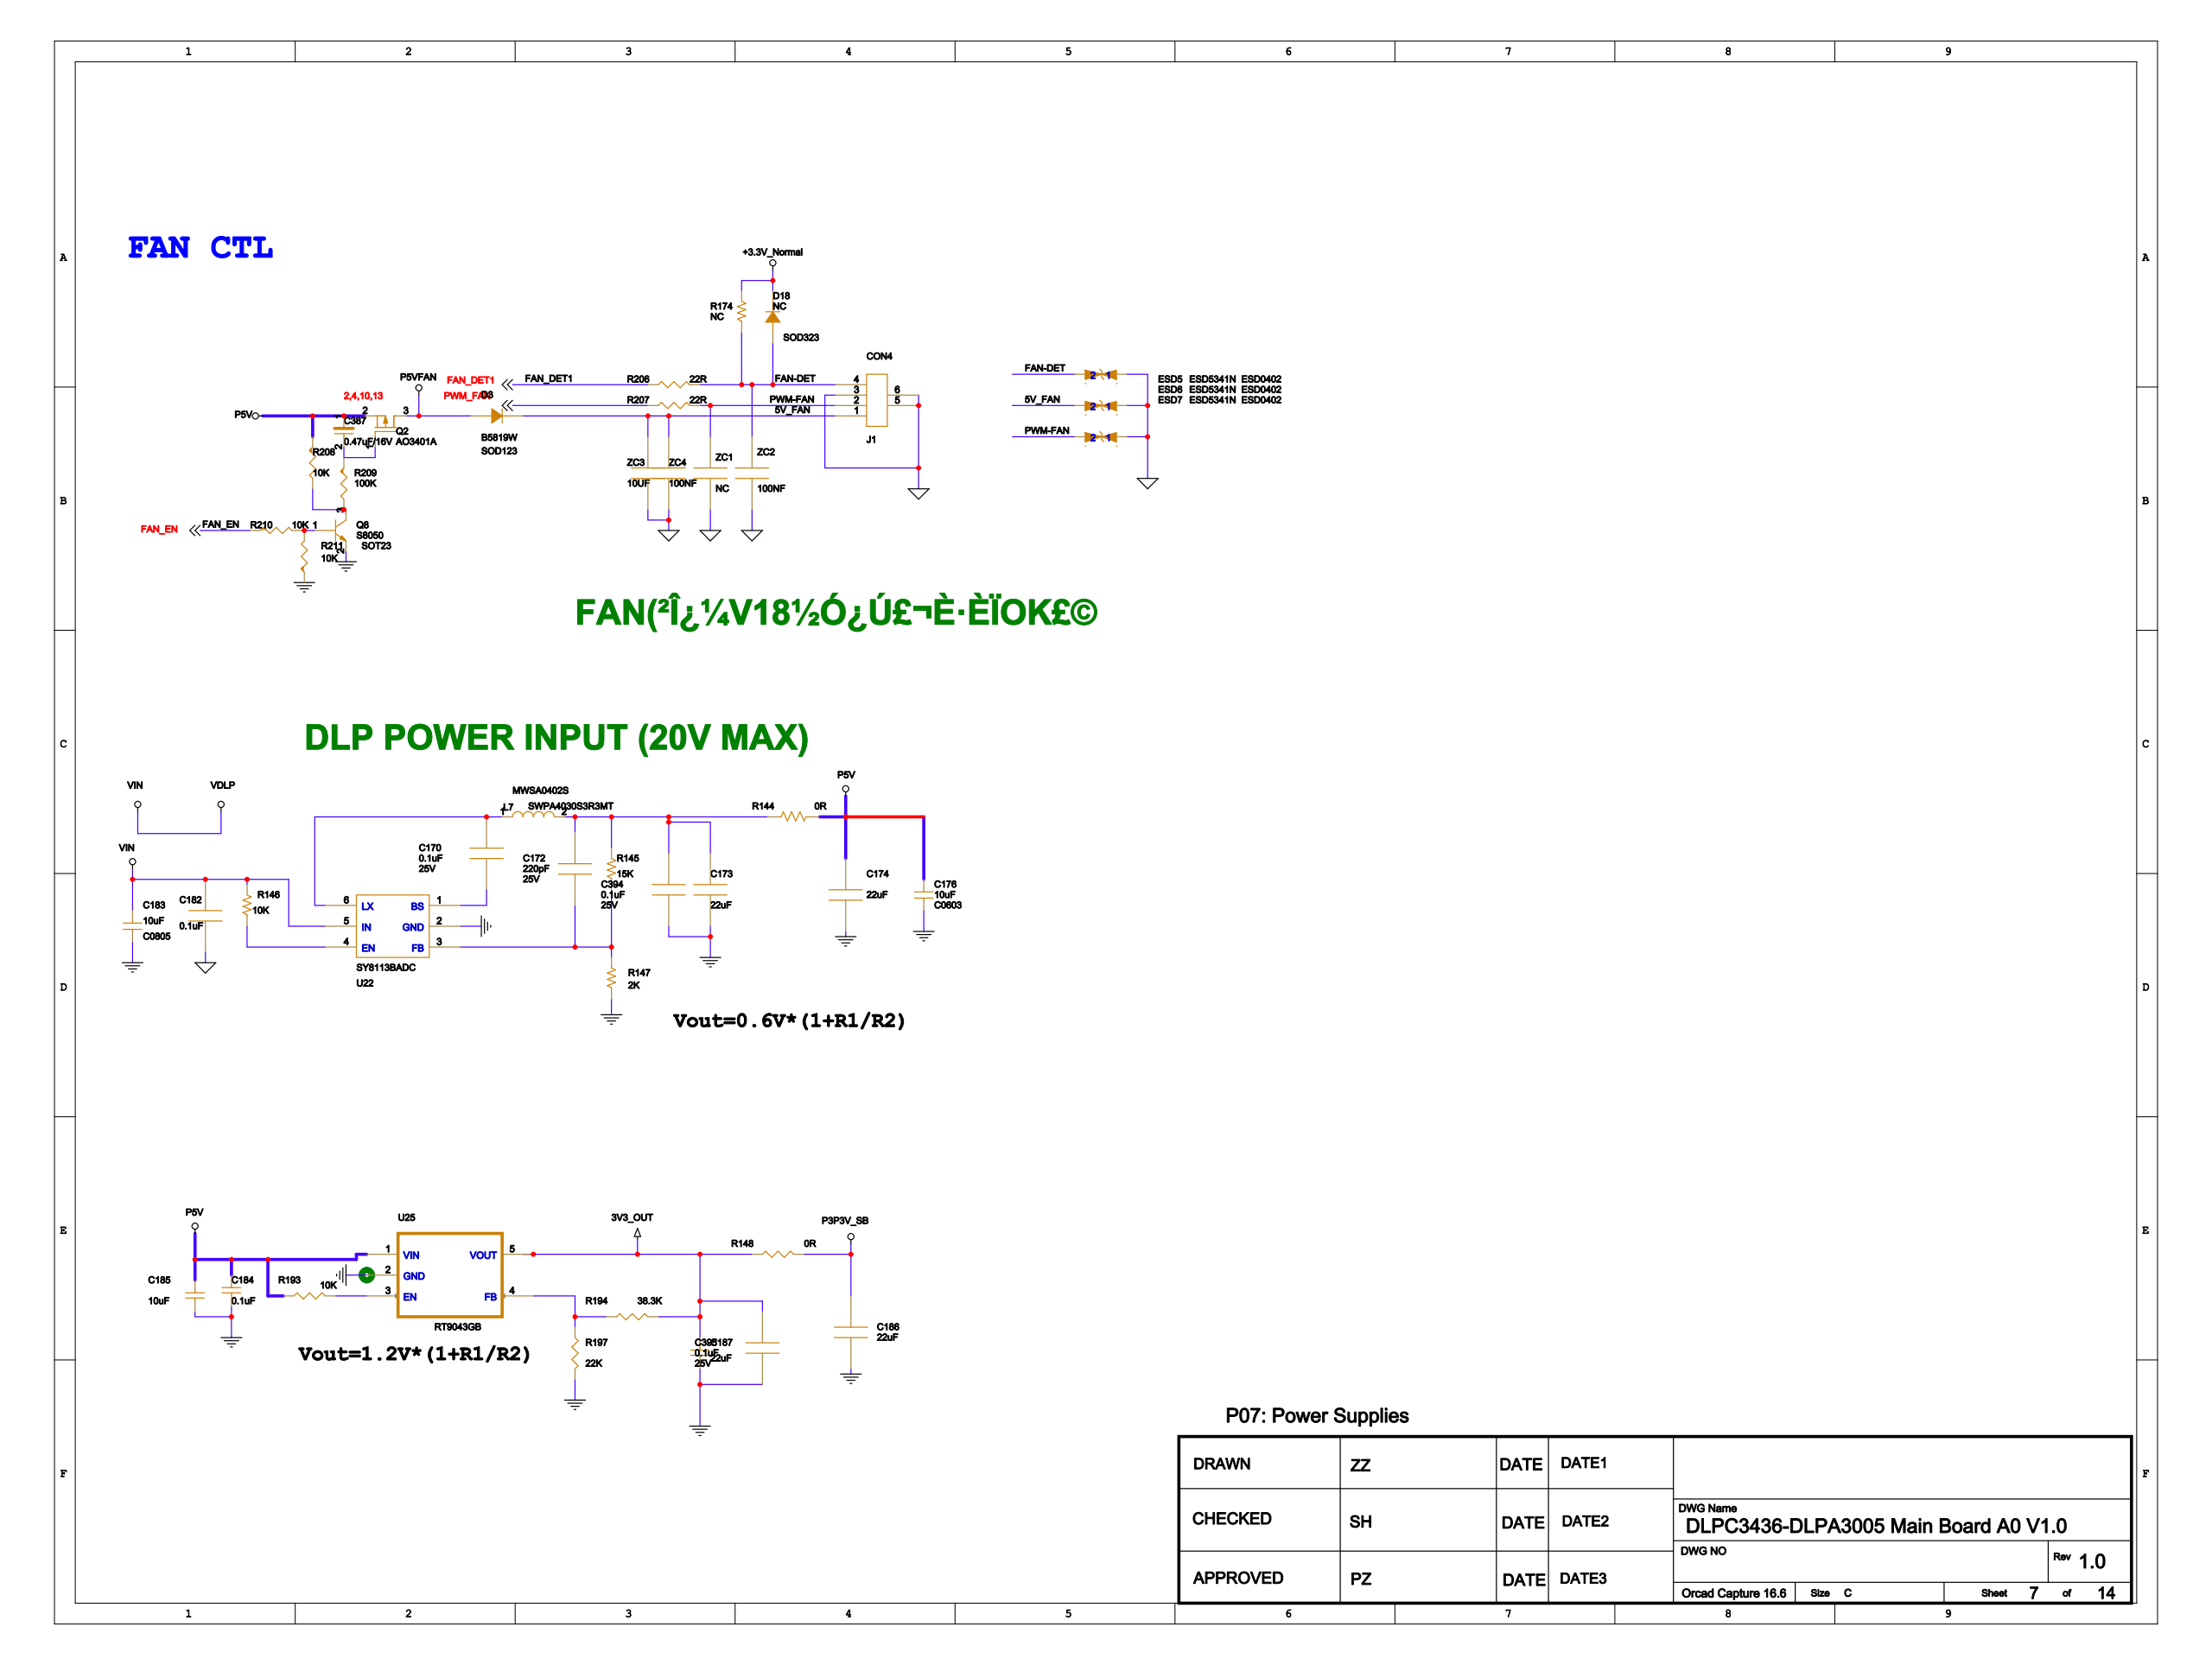Circuit board | Cadence Allegro | 1223 parts | 777 nets | one sheet of the schematic
Parts on this sheet (reference | value | footprint):
C170 | 0.1uF | C0402
C172 | 220pF | C0402
C173 | 22uF | C0603
C174 | 22uF | C0603
C176 | 10uF | C0603
C182 | 0.1uF | C0402
C183 | 10uF | C0805
C184 | 0.1uF | C0201
C185 | 10uF | C0603
C186 | 22uF | C0603
C187 | 22uF | C0603
C387 | 0.47uF/16V | C0402
C394 | 0.1uF | C0402
C395 | 0.1uF | C0402
D3 | B5819W | SOD123
D18 | NC | SOD323
ESD5 | ESD5341N | ESD0402
ESD6 | ESD5341N | ESD0402
ESD7 | ESD5341N | ESD0402
J1 | CON4 | CN1X4-1P25MM-WF
L7 | SWPA4030S3R3MT | MWSA0402S
Q2 | AO3401A | SOT23-100
Q8 | S8050 | SOT23
R144 | 0R | R0805
R145 | 15K | R0402
R146 | 10K | R0201
R147 | 2K | R0402
R148 | 0R | R0402
R174 | NC | R0402
R193 | 10K | R0201
R194 | 38.3K | R0402
R197 | 22K | R0402
R206 | 22R | R0402
R207 | 22R | R0402
R208 | 10K | R0402
R209 | 100K | R0402
R210 | 10K | R0402
R211 | 10K | R0402
U22 | SY8113BADC | SOT-23-6
U25 | RT9043GB | SOT25
ZC1 | NC | C0402
ZC2 | 100NF | C0402
ZC3 | 10uF | C0603
ZC4 | 100NF | C0402
Nets of these parts (net: part-pin ...):
GND: C173-2 C174-2 C176-1 C182-2 C183-1 C184-2 C185-2 C186-2 C187-2 C394-2 C395-2 ESD5-1 ESD6-1 ESD7-1 J1-3 J1-5 J1-6 Q8-2 R147-1 R197-2 R211-1 U22-2 U25-2 ZC1-1 ZC2-1 ZC3-1 ZC4-1
P3P3V_SB: C186-1 R148-2
VDLP: C182-1 C183-2 R146-2 U22-5
N23821148: C170-2 U22-1
N23821156: C170-1 L7-1 U22-6
N23821150: C172-1 C173-1 C394-1 L7-2 R144-1 R145-2
3V3_OUT: C187-1 C395-1 R148-1 R194-2 U25-5
+3.3V_EMMC: D18-2 R174-2
P5V: C174-1 C176-2 C184-1 C185-1 C387-1 Q2-2 R144-2 R193-1 R208-1 U25-1
N26081592: C387-2 Q2-1 R209-1
N23821152: C172-2 R145-1 R147-2 U22-3
5V_FAN: D3-2 ESD6-2 J1-1 ZC3-2 ZC4-2
FAN-DET: D18-1 ESD5-2 J1-4 R174-1 R206-2 ZC2-2
P5VFAN: D3-1 Q2-3
PWM-FAN: ESD7-2 J1-2 R207-2 ZC1-2
N26081662: Q8-1 R210-2 R211-2
N26081666: Q8-3 R208-2 R209-2
FAN_EN: R210-1
N23821144: R146-1 U22-4
N23963838: R193-2 U25-3
N23963921: R194-1 R197-1 U25-4
FAN_DET1: R206-1
PWM_FAN: R207-1